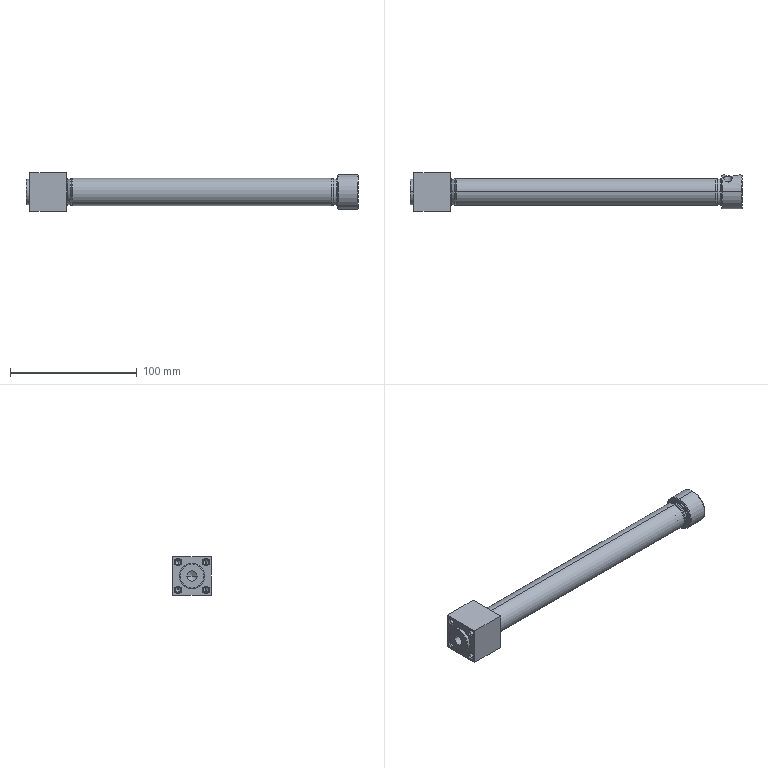Part | SolidWorks | features BaseBody 1 | 1 solid | 101 faces | box 262 x 30.5 x 30.5 mm | volume 46248 mm3 | cylinder 41 | cone 26 | plane 20 | torus 14 | commonest cylinder face diameters 4.134 x8 21.4 x6 3 x4 5.5 x4 8.566 x4 11 x4